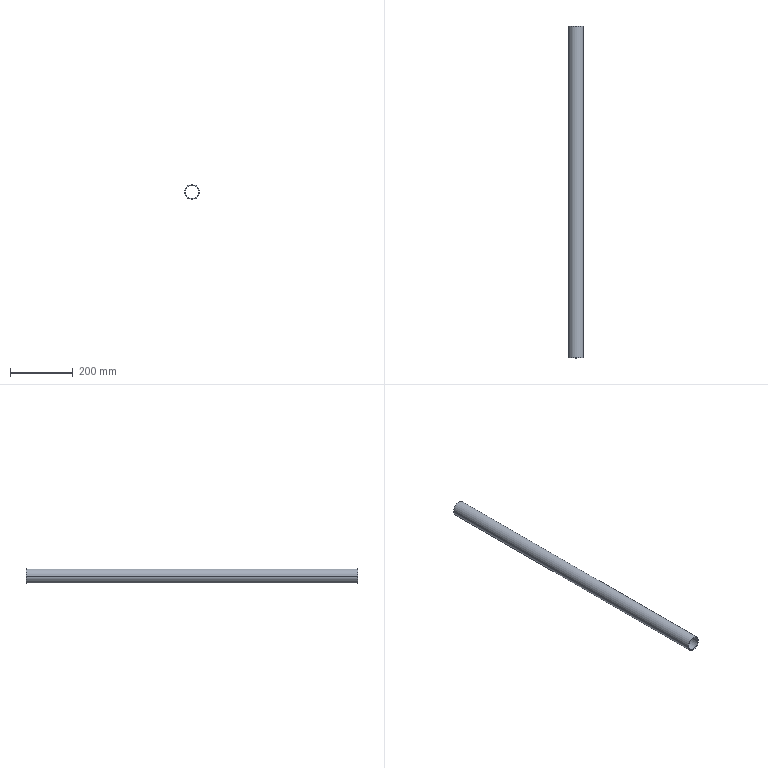Part | NX | 1 solid | 14 faces | box 47.8 x 1060 x 47.8 mm | volume 377061 mm3 | cone 8 | cylinder 4 | plane 2 | commonest cylinder face diameters 42.8 x2 47.8 x2
STEP:
#1=CARTESIAN_POINT('',(-166.15,-112.,-577.5));
#2=VERTEX_POINT('',#1);
#3=CARTESIAN_POINT('',(-123.35,-112.,-577.5));
#4=VERTEX_POINT('',#3);
#5=CARTESIAN_POINT('',(-144.75,-112.,-577.5));
#6=DIRECTION('',(0.,-1.,0.));
#7=DIRECTION('',(0.,0.,-1.));
#8=AXIS2_PLACEMENT_3D('',#5,#6,#7);
#9=CIRCLE('',#8,21.4);
#10=EDGE_CURVE('',#2,#4,#9,.T.);
#11=ORIENTED_EDGE('',*,*,#10,.T.);
#12=CARTESIAN_POINT('',(-123.35,947.,-577.5));
#13=VERTEX_POINT('',#12);
#14=CARTESIAN_POINT('',(-123.35,-100.5,-577.5));
#15=DIRECTION('',(0.,1.,0.));
#16=VECTOR('',#15,1000.);
#17=LINE('',#14,#16);
#18=EDGE_CURVE('',#13,#4,#17,.F.);
#19=ORIENTED_EDGE('',*,*,#18,.F.);
#20=CARTESIAN_POINT('',(-166.15,947.,-577.5));
#21=VERTEX_POINT('',#20);
#22=CARTESIAN_POINT('',(-144.75,947.,-577.5));
#23=DIRECTION('',(0.,1.,0.));
#24=DIRECTION('',(0.,0.,1.));
#25=AXIS2_PLACEMENT_3D('',#22,#23,#24);
#26=CIRCLE('',#25,21.4);
#27=EDGE_CURVE('',#13,#21,#26,.T.);
#28=ORIENTED_EDGE('',*,*,#27,.T.);
#29=CARTESIAN_POINT('',(-166.15,-100.5,-577.5));
#30=DIRECTION('',(0.,1.,0.));
#31=VECTOR('',#30,1000.);
#32=LINE('',#29,#31);
#33=EDGE_CURVE('',#21,#2,#32,.F.);
#34=ORIENTED_EDGE('',*,*,#33,.T.);
#35=EDGE_LOOP('',(#11,#19,#28,#34));
#36=FACE_BOUND('',#35,.T.);
#37=CARTESIAN_POINT('',(-144.75,-100.5,-577.5));
#38=DIRECTION('',(0.,1.,0.));
#39=DIRECTION('',(-1.,0.,0.));
#40=AXIS2_PLACEMENT_3D('',#37,#38,#39);
#41=CYLINDRICAL_SURFACE('',#40,21.4);
#42=ADVANCED_FACE('',(#36),#41,.F.);
#43=CARTESIAN_POINT('',(-120.85,947.,-577.5));
#44=VERTEX_POINT('',#43);
#45=CARTESIAN_POINT('',(-168.65,947.,-577.5));
#46=VERTEX_POINT('',#45);
#47=CARTESIAN_POINT('',(-144.75,947.,-577.5));
#48=DIRECTION('',(0.,-1.,0.));
#49=DIRECTION('',(0.,0.,-1.));
#50=AXIS2_PLACEMENT_3D('',#47,#48,#49);
#51=CIRCLE('',#50,23.9);
#52=EDGE_CURVE('',#44,#46,#51,.T.);
#53=ORIENTED_EDGE('',*,*,#52,.T.);
#54=CARTESIAN_POINT('',(-168.65,-112.,-577.5));
#55=VERTEX_POINT('',#54);
#56=CARTESIAN_POINT('',(-168.65,-100.5,-577.5));
#57=DIRECTION('',(0.,1.,0.));
#58=VECTOR('',#57,1000.);
#59=LINE('',#56,#58);
#60=EDGE_CURVE('',#46,#55,#59,.F.);
#61=ORIENTED_EDGE('',*,*,#60,.T.);
#62=CARTESIAN_POINT('',(-120.85,-112.,-577.5));
#63=VERTEX_POINT('',#62);
#64=CARTESIAN_POINT('',(-144.75,-112.,-577.5));
#65=DIRECTION('',(0.,1.,0.));
#66=DIRECTION('',(0.,0.,1.));
#67=AXIS2_PLACEMENT_3D('',#64,#65,#66);
#68=CIRCLE('',#67,23.9);
#69=EDGE_CURVE('',#55,#63,#68,.T.);
#70=ORIENTED_EDGE('',*,*,#69,.T.);
#71=CARTESIAN_POINT('',(-120.85,-100.5,-577.5));
#72=DIRECTION('',(0.,1.,0.));
#73=VECTOR('',#72,1000.);
#74=LINE('',#71,#73);
#75=EDGE_CURVE('',#44,#63,#74,.F.);
#76=ORIENTED_EDGE('',*,*,#75,.F.);
#77=EDGE_LOOP('',(#53,#61,#70,#76));
#78=FACE_BOUND('',#77,.T.);
#79=CARTESIAN_POINT('',(-144.75,-100.5,-577.5));
#80=DIRECTION('',(0.,1.,0.));
#81=DIRECTION('',(-1.,0.,0.));
#82=AXIS2_PLACEMENT_3D('',#79,#80,#81);
#83=CYLINDRICAL_SURFACE('',#82,23.9);
#84=ADVANCED_FACE('',(#78),#83,.T.);
#85=CARTESIAN_POINT('',(-121.35,947.5,-577.5));
#86=VERTEX_POINT('',#85);
#87=CARTESIAN_POINT('',(-168.15,947.5,-577.5));
#88=VERTEX_POINT('',#87);
#89=CARTESIAN_POINT('',(-144.75,947.5,-577.5));
#90=DIRECTION('',(0.,-1.,0.));
#91=DIRECTION('',(0.,0.,-1.));
#92=AXIS2_PLACEMENT_3D('',#89,#90,#91);
#93=CIRCLE('',#92,23.4);
#94=EDGE_CURVE('',#86,#88,#93,.T.);
#95=ORIENTED_EDGE('',*,*,#94,.F.);
#96=CARTESIAN_POINT('',(-144.75,947.5,-577.5));
#97=DIRECTION('',(0.,-1.,0.));
#98=DIRECTION('',(0.,0.,-1.));
#99=AXIS2_PLACEMENT_3D('',#96,#97,#98);
#100=CIRCLE('',#99,23.4);
#101=EDGE_CURVE('',#88,#86,#100,.T.);
#102=ORIENTED_EDGE('',*,*,#101,.F.);
#103=EDGE_LOOP('',(#95,#102));
#104=FACE_BOUND('',#103,.T.);
#105=CARTESIAN_POINT('',(-166.65,947.5,-577.5));
#106=VERTEX_POINT('',#105);
#107=CARTESIAN_POINT('',(-122.85,947.5,-577.5));
#108=VERTEX_POINT('',#107);
#109=CARTESIAN_POINT('',(-144.75,947.5,-577.5));
#110=DIRECTION('',(0.,1.,0.));
#111=DIRECTION('',(0.,0.,1.));
#112=AXIS2_PLACEMENT_3D('',#109,#110,#111);
#113=CIRCLE('',#112,21.9);
#114=EDGE_CURVE('',#106,#108,#113,.T.);
#115=ORIENTED_EDGE('',*,*,#114,.F.);
#116=CARTESIAN_POINT('',(-144.75,947.5,-577.5));
#117=DIRECTION('',(0.,1.,0.));
#118=DIRECTION('',(0.,0.,1.));
#119=AXIS2_PLACEMENT_3D('',#116,#117,#118);
#120=CIRCLE('',#119,21.9);
#121=EDGE_CURVE('',#108,#106,#120,.T.);
#122=ORIENTED_EDGE('',*,*,#121,.F.);
#123=EDGE_LOOP('',(#115,#122));
#124=FACE_BOUND('',#123,.T.);
#125=CARTESIAN_POINT('',(-49.,947.5,-637.5));
#126=DIRECTION('',(0.,1.,0.));
#127=DIRECTION('',(1.,0.,0.));
#128=AXIS2_PLACEMENT_3D('',#125,#126,#127);
#129=PLANE('',#128);
#130=ADVANCED_FACE('',(#104,#124),#129,.T.);
#131=ORIENTED_EDGE('',*,*,#52,.F.);
#132=CARTESIAN_POINT('',(-121.35,947.5,-577.5));
#133=DIRECTION('',(0.7071,-0.7071,0.));
#134=VECTOR('',#133,1000.);
#135=LINE('',#132,#134);
#136=EDGE_CURVE('',#44,#86,#135,.F.);
#137=ORIENTED_EDGE('',*,*,#136,.T.);
#138=ORIENTED_EDGE('',*,*,#94,.T.);
#139=CARTESIAN_POINT('',(-168.15,947.5,-577.5));
#140=DIRECTION('',(-0.7071,-0.7071,0.));
#141=VECTOR('',#140,1000.);
#142=LINE('',#139,#141);
#143=EDGE_CURVE('',#46,#88,#142,.F.);
#144=ORIENTED_EDGE('',*,*,#143,.F.);
#145=EDGE_LOOP('',(#131,#137,#138,#144));
#146=FACE_BOUND('',#145,.T.);
#147=CARTESIAN_POINT('',(-144.75,947.5,-577.5));
#148=DIRECTION('',(0.,-1.,0.));
#149=DIRECTION('',(-1.,0.,0.));
#150=AXIS2_PLACEMENT_3D('',#147,#148,#149);
#151=CONICAL_SURFACE('',#150,23.4,0.7854);
#152=ADVANCED_FACE('',(#146),#151,.T.);
#153=ORIENTED_EDGE('',*,*,#27,.F.);
#154=CARTESIAN_POINT('',(-122.85,947.5,-577.5));
#155=DIRECTION('',(0.7071,0.7071,0.));
#156=VECTOR('',#155,1000.);
#157=LINE('',#154,#156);
#158=EDGE_CURVE('',#13,#108,#157,.T.);
#159=ORIENTED_EDGE('',*,*,#158,.T.);
#160=ORIENTED_EDGE('',*,*,#121,.T.);
#161=CARTESIAN_POINT('',(-166.65,947.5,-577.5));
#162=DIRECTION('',(-0.7071,0.7071,0.));
#163=VECTOR('',#162,1000.);
#164=LINE('',#161,#163);
#165=EDGE_CURVE('',#21,#106,#164,.T.);
#166=ORIENTED_EDGE('',*,*,#165,.F.);
#167=EDGE_LOOP('',(#153,#159,#160,#166));
#168=FACE_BOUND('',#167,.T.);
#169=CARTESIAN_POINT('',(-144.75,947.5,-577.5));
#170=DIRECTION('',(0.,1.,0.));
#171=DIRECTION('',(1.,0.,0.));
#172=AXIS2_PLACEMENT_3D('',#169,#170,#171);
#173=CONICAL_SURFACE('',#172,21.9,0.7854);
#174=ADVANCED_FACE('',(#168),#173,.F.);
#175=CARTESIAN_POINT('',(-121.35,-112.5,-577.5));
#176=VERTEX_POINT('',#175);
#177=CARTESIAN_POINT('',(-168.15,-112.5,-577.5));
#178=VERTEX_POINT('',#177);
#179=CARTESIAN_POINT('',(-144.75,-112.5,-577.5));
#180=DIRECTION('',(0.,1.,0.));
#181=DIRECTION('',(0.,0.,1.));
#182=AXIS2_PLACEMENT_3D('',#179,#180,#181);
#183=CIRCLE('',#182,23.4);
#184=EDGE_CURVE('',#176,#178,#183,.T.);
#185=ORIENTED_EDGE('',*,*,#184,.T.);
#186=CARTESIAN_POINT('',(-168.65,-112.,-577.5));
#187=DIRECTION('',(-0.7071,0.7071,0.));
#188=VECTOR('',#187,1000.);
#189=LINE('',#186,#188);
#190=EDGE_CURVE('',#55,#178,#189,.F.);
#191=ORIENTED_EDGE('',*,*,#190,.F.);
#192=CARTESIAN_POINT('',(-144.75,-112.,-577.5));
#193=DIRECTION('',(0.,1.,0.));
#194=DIRECTION('',(0.,0.,1.));
#195=AXIS2_PLACEMENT_3D('',#192,#193,#194);
#196=CIRCLE('',#195,23.9);
#197=EDGE_CURVE('',#63,#55,#196,.T.);
#198=ORIENTED_EDGE('',*,*,#197,.F.);
#199=CARTESIAN_POINT('',(-120.85,-112.,-577.5));
#200=DIRECTION('',(0.7071,0.7071,0.));
#201=VECTOR('',#200,1000.);
#202=LINE('',#199,#201);
#203=EDGE_CURVE('',#63,#176,#202,.F.);
#204=ORIENTED_EDGE('',*,*,#203,.T.);
#205=EDGE_LOOP('',(#185,#191,#198,#204));
#206=FACE_BOUND('',#205,.T.);
#207=CARTESIAN_POINT('',(-144.75,-112.,-577.5));
#208=DIRECTION('',(0.,1.,0.));
#209=DIRECTION('',(1.,0.,0.));
#210=AXIS2_PLACEMENT_3D('',#207,#208,#209);
#211=CONICAL_SURFACE('',#210,23.9,0.7854);
#212=ADVANCED_FACE('',(#206),#211,.T.);
#213=CARTESIAN_POINT('',(-122.85,-112.5,-577.5));
#214=VERTEX_POINT('',#213);
#215=CARTESIAN_POINT('',(-166.65,-112.5,-577.5));
#216=VERTEX_POINT('',#215);
#217=CARTESIAN_POINT('',(-144.75,-112.5,-577.5));
#218=DIRECTION('',(0.,-1.,0.));
#219=DIRECTION('',(0.,0.,-1.));
#220=AXIS2_PLACEMENT_3D('',#217,#218,#219);
#221=CIRCLE('',#220,21.9);
#222=EDGE_CURVE('',#214,#216,#221,.T.);
#223=ORIENTED_EDGE('',*,*,#222,.T.);
#224=CARTESIAN_POINT('',(-166.65,-112.5,-577.5));
#225=DIRECTION('',(-0.7071,-0.7071,0.));
#226=VECTOR('',#225,1000.);
#227=LINE('',#224,#226);
#228=EDGE_CURVE('',#216,#2,#227,.F.);
#229=ORIENTED_EDGE('',*,*,#228,.T.);
#230=CARTESIAN_POINT('',(-144.75,-112.,-577.5));
#231=DIRECTION('',(0.,-1.,0.));
#232=DIRECTION('',(0.,0.,-1.));
#233=AXIS2_PLACEMENT_3D('',#230,#231,#232);
#234=CIRCLE('',#233,21.4);
#235=EDGE_CURVE('',#4,#2,#234,.T.);
#236=ORIENTED_EDGE('',*,*,#235,.F.);
#237=CARTESIAN_POINT('',(-122.85,-112.5,-577.5));
#238=DIRECTION('',(0.7071,-0.7071,0.));
#239=VECTOR('',#238,1000.);
#240=LINE('',#237,#239);
#241=EDGE_CURVE('',#214,#4,#240,.F.);
#242=ORIENTED_EDGE('',*,*,#241,.F.);
#243=EDGE_LOOP('',(#223,#229,#236,#242));
#244=FACE_BOUND('',#243,.T.);
#245=CARTESIAN_POINT('',(-144.75,-112.5,-577.5));
#246=DIRECTION('',(0.,-1.,0.));
#247=DIRECTION('',(-1.,0.,0.));
#248=AXIS2_PLACEMENT_3D('',#245,#246,#247);
#249=CONICAL_SURFACE('',#248,21.9,0.7854);
#250=ADVANCED_FACE('',(#244),#249,.F.);
#251=ORIENTED_EDGE('',*,*,#184,.F.);
#252=CARTESIAN_POINT('',(-144.75,-112.5,-577.5));
#253=DIRECTION('',(0.,1.,0.));
#254=DIRECTION('',(0.,0.,1.));
#255=AXIS2_PLACEMENT_3D('',#252,#253,#254);
#256=CIRCLE('',#255,23.4);
#257=EDGE_CURVE('',#178,#176,#256,.T.);
#258=ORIENTED_EDGE('',*,*,#257,.F.);
#259=EDGE_LOOP('',(#251,#258));
#260=FACE_BOUND('',#259,.T.);
#261=ORIENTED_EDGE('',*,*,#222,.F.);
#262=CARTESIAN_POINT('',(-144.75,-112.5,-577.5));
#263=DIRECTION('',(0.,-1.,0.));
#264=DIRECTION('',(0.,0.,-1.));
#265=AXIS2_PLACEMENT_3D('',#262,#263,#264);
#266=CIRCLE('',#265,21.9);
#267=EDGE_CURVE('',#216,#214,#266,.T.);
#268=ORIENTED_EDGE('',*,*,#267,.F.);
#269=EDGE_LOOP('',(#261,#268));
#270=FACE_BOUND('',#269,.T.);
#271=CARTESIAN_POINT('',(-144.75,-112.5,-710.75));
#272=DIRECTION('',(0.,1.,0.));
#273=DIRECTION('',(1.,0.,0.));
#274=AXIS2_PLACEMENT_3D('',#271,#272,#273);
#275=PLANE('',#274);
#276=ADVANCED_FACE('',(#260,#270),#275,.F.);
#277=ORIENTED_EDGE('',*,*,#143,.T.);
#278=ORIENTED_EDGE('',*,*,#101,.T.);
#279=ORIENTED_EDGE('',*,*,#136,.F.);
#280=CARTESIAN_POINT('',(-144.75,947.,-577.5));
#281=DIRECTION('',(0.,-1.,0.));
#282=DIRECTION('',(0.,0.,-1.));
#283=AXIS2_PLACEMENT_3D('',#280,#281,#282);
#284=CIRCLE('',#283,23.9);
#285=EDGE_CURVE('',#46,#44,#284,.T.);
#286=ORIENTED_EDGE('',*,*,#285,.F.);
#287=EDGE_LOOP('',(#277,#278,#279,#286));
#288=FACE_BOUND('',#287,.T.);
#289=CARTESIAN_POINT('',(-144.75,947.5,-577.5));
#290=DIRECTION('',(0.,-1.,0.));
#291=DIRECTION('',(-1.,0.,0.));
#292=AXIS2_PLACEMENT_3D('',#289,#290,#291);
#293=CONICAL_SURFACE('',#292,23.4,0.7854);
#294=ADVANCED_FACE('',(#288),#293,.T.);
#295=ORIENTED_EDGE('',*,*,#60,.F.);
#296=ORIENTED_EDGE('',*,*,#285,.T.);
#297=ORIENTED_EDGE('',*,*,#75,.T.);
#298=ORIENTED_EDGE('',*,*,#197,.T.);
#299=EDGE_LOOP('',(#295,#296,#297,#298));
#300=FACE_BOUND('',#299,.T.);
#301=CARTESIAN_POINT('',(-144.75,-100.5,-577.5));
#302=DIRECTION('',(0.,1.,0.));
#303=DIRECTION('',(-1.,0.,0.));
#304=AXIS2_PLACEMENT_3D('',#301,#302,#303);
#305=CYLINDRICAL_SURFACE('',#304,23.9);
#306=ADVANCED_FACE('',(#300),#305,.T.);
#307=ORIENTED_EDGE('',*,*,#69,.F.);
#308=ORIENTED_EDGE('',*,*,#190,.T.);
#309=ORIENTED_EDGE('',*,*,#257,.T.);
#310=ORIENTED_EDGE('',*,*,#203,.F.);
#311=EDGE_LOOP('',(#307,#308,#309,#310));
#312=FACE_BOUND('',#311,.T.);
#313=CARTESIAN_POINT('',(-144.75,-112.,-577.5));
#314=DIRECTION('',(0.,1.,0.));
#315=DIRECTION('',(1.,0.,0.));
#316=AXIS2_PLACEMENT_3D('',#313,#314,#315);
#317=CONICAL_SURFACE('',#316,23.9,0.7854);
#318=ADVANCED_FACE('',(#312),#317,.T.);
#319=ORIENTED_EDGE('',*,*,#10,.F.);
#320=ORIENTED_EDGE('',*,*,#228,.F.);
#321=ORIENTED_EDGE('',*,*,#267,.T.);
#322=ORIENTED_EDGE('',*,*,#241,.T.);
#323=EDGE_LOOP('',(#319,#320,#321,#322));
#324=FACE_BOUND('',#323,.T.);
#325=CARTESIAN_POINT('',(-144.75,-112.5,-577.5));
#326=DIRECTION('',(0.,-1.,0.));
#327=DIRECTION('',(-1.,0.,0.));
#328=AXIS2_PLACEMENT_3D('',#325,#326,#327);
#329=CONICAL_SURFACE('',#328,21.9,0.7854);
#330=ADVANCED_FACE('',(#324),#329,.F.);
#331=ORIENTED_EDGE('',*,*,#114,.T.);
#332=ORIENTED_EDGE('',*,*,#158,.F.);
#333=CARTESIAN_POINT('',(-144.75,947.,-577.5));
#334=DIRECTION('',(0.,1.,0.));
#335=DIRECTION('',(0.,0.,1.));
#336=AXIS2_PLACEMENT_3D('',#333,#334,#335);
#337=CIRCLE('',#336,21.4);
#338=EDGE_CURVE('',#21,#13,#337,.T.);
#339=ORIENTED_EDGE('',*,*,#338,.F.);
#340=ORIENTED_EDGE('',*,*,#165,.T.);
#341=EDGE_LOOP('',(#331,#332,#339,#340));
#342=FACE_BOUND('',#341,.T.);
#343=CARTESIAN_POINT('',(-144.75,947.5,-577.5));
#344=DIRECTION('',(0.,1.,0.));
#345=DIRECTION('',(1.,0.,0.));
#346=AXIS2_PLACEMENT_3D('',#343,#344,#345);
#347=CONICAL_SURFACE('',#346,21.9,0.7854);
#348=ADVANCED_FACE('',(#342),#347,.F.);
#349=ORIENTED_EDGE('',*,*,#33,.F.);
#350=ORIENTED_EDGE('',*,*,#338,.T.);
#351=ORIENTED_EDGE('',*,*,#18,.T.);
#352=ORIENTED_EDGE('',*,*,#235,.T.);
#353=EDGE_LOOP('',(#349,#350,#351,#352));
#354=FACE_BOUND('',#353,.T.);
#355=CARTESIAN_POINT('',(-144.75,-100.5,-577.5));
#356=DIRECTION('',(0.,1.,0.));
#357=DIRECTION('',(-1.,0.,0.));
#358=AXIS2_PLACEMENT_3D('',#355,#356,#357);
#359=CYLINDRICAL_SURFACE('',#358,21.4);
#360=ADVANCED_FACE('',(#354),#359,.F.);
#361=CLOSED_SHELL('',(#42,#84,#130,#152,#174,#212,#250,#276,#294,#306,#318,#330,#348,#360));
#362=MANIFOLD_SOLID_BREP('',#361);
#363=(LENGTH_UNIT()NAMED_UNIT(*)SI_UNIT(.MILLI.,.METRE.));
#364=UNCERTAINTY_MEASURE_WITH_UNIT(LENGTH_MEASURE(0.00001),#363,'','');
#365=(NAMED_UNIT(*)PLANE_ANGLE_UNIT()SI_UNIT($,.RADIAN.));
#366=(NAMED_UNIT(*)SI_UNIT($,.STERADIAN.)SOLID_ANGLE_UNIT());
#367=(GEOMETRIC_REPRESENTATION_CONTEXT(3)GLOBAL_UNCERTAINTY_ASSIGNED_CONTEXT((#364))GLOBAL_UNIT_ASSIGNED_CONTEXT((#363,#365,#366))REPRESENTATION_CONTEXT('',''));
#368=ADVANCED_BREP_SHAPE_REPRESENTATION('',(#362),#367);